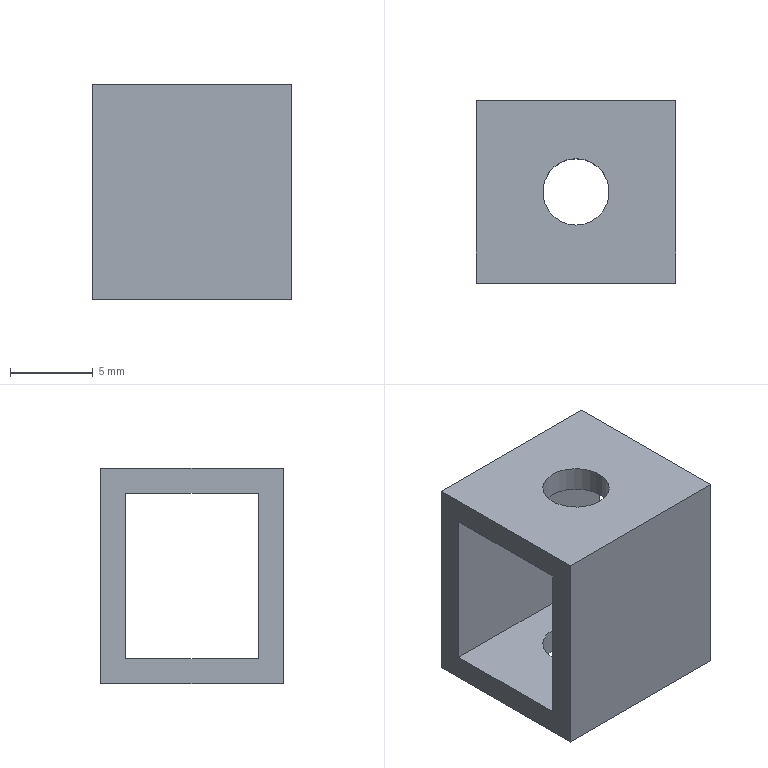Part | STEP file | 1-54.2 | 1 solid | 12 faces | box 12 x 11 x 13 mm | volume 718.301 mm3 | plane 10 | cylinder 2 | commonest cylinder face diameters 4 x2
STEP:
#1=CARTESIAN_POINT('',(0.,0.,0.));
#2=DIRECTION('',(0.,0.,1.));
#3=DIRECTION('',(1.,0.,0.));
#4=AXIS2_PLACEMENT_3D('',#1,#2,#3);
#5=CARTESIAN_POINT('',(6.,-5.5,-6.5));
#6=VERTEX_POINT('',#5);
#7=CARTESIAN_POINT('',(6.,5.5,-6.5));
#8=VERTEX_POINT('',#7);
#9=CARTESIAN_POINT('',(6.,-5.5,-6.5));
#10=DIRECTION('',(0.,1.,0.));
#11=VECTOR('',#10,1.);
#12=LINE('',#9,#11);
#13=CARTESIAN_POINT('',(6.,1.,0.));
#14=DIRECTION('',(1.,0.,0.));
#15=DIRECTION('',(0.,1.,0.));
#16=AXIS2_PLACEMENT_3D('',#13,#14,#15);
#17=PLANE('',#16);
#18=CARTESIAN_POINT('',(-6.5,-6.5));
#19=DIRECTION('',(1.,0.));
#20=VECTOR('',#19,1.);
#21=LINE('',#18,#20);
#22=(GEOMETRIC_REPRESENTATION_CONTEXT(2)PARAMETRIC_REPRESENTATION_CONTEXT()REPRESENTATION_CONTEXT('',''));
#23=DEFINITIONAL_REPRESENTATION('',(#21),#22);
#24=PCURVE('',#17,#23);
#25=CARTESIAN_POINT('',(0.,0.,-6.5));
#26=DIRECTION('',(0.,0.,1.));
#27=DIRECTION('',(0.,1.,0.));
#28=AXIS2_PLACEMENT_3D('',#25,#26,#27);
#29=PLANE('',#28);
#30=CARTESIAN_POINT('',(-5.5,-6.));
#31=DIRECTION('',(1.,0.));
#32=VECTOR('',#31,1.);
#33=LINE('',#30,#32);
#34=(GEOMETRIC_REPRESENTATION_CONTEXT(2)PARAMETRIC_REPRESENTATION_CONTEXT()REPRESENTATION_CONTEXT('',''));
#35=DEFINITIONAL_REPRESENTATION('',(#33),#34);
#36=PCURVE('',#29,#35);
#37=SURFACE_CURVE('',#12,(#24,#36),.PCURVE_S1.);
#38=EDGE_CURVE('',#6,#8,#37,.T.);
#39=ORIENTED_EDGE('',*,*,#38,.T.);
#40=CARTESIAN_POINT('',(6.,5.5,6.5));
#41=VERTEX_POINT('',#40);
#42=CARTESIAN_POINT('',(6.,5.5,-6.5));
#43=DIRECTION('',(0.,0.,1.));
#44=VECTOR('',#43,1.);
#45=LINE('',#42,#44);
#46=CARTESIAN_POINT('',(4.5,-6.5));
#47=DIRECTION('',(0.,1.));
#48=VECTOR('',#47,1.);
#49=LINE('',#46,#48);
#50=(GEOMETRIC_REPRESENTATION_CONTEXT(2)PARAMETRIC_REPRESENTATION_CONTEXT()REPRESENTATION_CONTEXT('',''));
#51=DEFINITIONAL_REPRESENTATION('',(#49),#50);
#52=PCURVE('',#17,#51);
#53=CARTESIAN_POINT('',(0.,5.5,0.));
#54=DIRECTION('',(0.,-1.,0.));
#55=DIRECTION('',(0.,0.,1.));
#56=AXIS2_PLACEMENT_3D('',#53,#54,#55);
#57=PLANE('',#56);
#58=CARTESIAN_POINT('',(-6.5,-6.));
#59=DIRECTION('',(1.,0.));
#60=VECTOR('',#59,1.);
#61=LINE('',#58,#60);
#62=(GEOMETRIC_REPRESENTATION_CONTEXT(2)PARAMETRIC_REPRESENTATION_CONTEXT()REPRESENTATION_CONTEXT('',''));
#63=DEFINITIONAL_REPRESENTATION('',(#61),#62);
#64=PCURVE('',#57,#63);
#65=SURFACE_CURVE('',#45,(#52,#64),.PCURVE_S1.);
#66=EDGE_CURVE('',#8,#41,#65,.T.);
#67=ORIENTED_EDGE('',*,*,#66,.T.);
#68=CARTESIAN_POINT('',(6.,-5.5,6.5));
#69=VERTEX_POINT('',#68);
#70=CARTESIAN_POINT('',(6.,5.5,6.5));
#71=DIRECTION('',(0.,-1.,0.));
#72=VECTOR('',#71,1.);
#73=LINE('',#70,#72);
#74=CARTESIAN_POINT('',(4.5,6.5));
#75=DIRECTION('',(-1.,0.));
#76=VECTOR('',#75,1.);
#77=LINE('',#74,#76);
#78=(GEOMETRIC_REPRESENTATION_CONTEXT(2)PARAMETRIC_REPRESENTATION_CONTEXT()REPRESENTATION_CONTEXT('',''));
#79=DEFINITIONAL_REPRESENTATION('',(#77),#78);
#80=PCURVE('',#17,#79);
#81=CARTESIAN_POINT('',(0.,0.,6.5));
#82=DIRECTION('',(0.,0.,-1.));
#83=DIRECTION('',(0.,-1.,0.));
#84=AXIS2_PLACEMENT_3D('',#81,#82,#83);
#85=PLANE('',#84);
#86=CARTESIAN_POINT('',(-5.5,-6.));
#87=DIRECTION('',(1.,0.));
#88=VECTOR('',#87,1.);
#89=LINE('',#86,#88);
#90=(GEOMETRIC_REPRESENTATION_CONTEXT(2)PARAMETRIC_REPRESENTATION_CONTEXT()REPRESENTATION_CONTEXT('',''));
#91=DEFINITIONAL_REPRESENTATION('',(#89),#90);
#92=PCURVE('',#85,#91);
#93=SURFACE_CURVE('',#73,(#80,#92),.PCURVE_S1.);
#94=EDGE_CURVE('',#41,#69,#93,.T.);
#95=ORIENTED_EDGE('',*,*,#94,.T.);
#96=CARTESIAN_POINT('',(6.,-5.5,6.5));
#97=DIRECTION('',(0.,0.,-1.));
#98=VECTOR('',#97,1.);
#99=LINE('',#96,#98);
#100=CARTESIAN_POINT('',(-6.5,6.5));
#101=DIRECTION('',(0.,-1.));
#102=VECTOR('',#101,1.);
#103=LINE('',#100,#102);
#104=(GEOMETRIC_REPRESENTATION_CONTEXT(2)PARAMETRIC_REPRESENTATION_CONTEXT()REPRESENTATION_CONTEXT('',''));
#105=DEFINITIONAL_REPRESENTATION('',(#103),#104);
#106=PCURVE('',#17,#105);
#107=CARTESIAN_POINT('',(0.,-5.5,0.));
#108=DIRECTION('',(0.,1.,0.));
#109=DIRECTION('',(0.,0.,-1.));
#110=AXIS2_PLACEMENT_3D('',#107,#108,#109);
#111=PLANE('',#110);
#112=CARTESIAN_POINT('',(-6.5,-6.));
#113=DIRECTION('',(1.,0.));
#114=VECTOR('',#113,1.);
#115=LINE('',#112,#114);
#116=(GEOMETRIC_REPRESENTATION_CONTEXT(2)PARAMETRIC_REPRESENTATION_CONTEXT()REPRESENTATION_CONTEXT('',''));
#117=DEFINITIONAL_REPRESENTATION('',(#115),#116);
#118=PCURVE('',#111,#117);
#119=SURFACE_CURVE('',#99,(#106,#118),.PCURVE_S1.);
#120=EDGE_CURVE('',#69,#6,#119,.T.);
#121=ORIENTED_EDGE('',*,*,#120,.T.);
#122=EDGE_LOOP('',(#39,#67,#95,#121));
#123=FACE_BOUND('',#122,.T.);
#124=CARTESIAN_POINT('',(6.,-4.,-5.));
#125=VERTEX_POINT('',#124);
#126=CARTESIAN_POINT('',(6.,-4.,5.));
#127=VERTEX_POINT('',#126);
#128=CARTESIAN_POINT('',(6.,-4.,-5.));
#129=DIRECTION('',(0.,0.,1.));
#130=VECTOR('',#129,1.);
#131=LINE('',#128,#130);
#132=CARTESIAN_POINT('',(-5.,-5.));
#133=DIRECTION('',(0.,1.));
#134=VECTOR('',#133,1.);
#135=LINE('',#132,#134);
#136=(GEOMETRIC_REPRESENTATION_CONTEXT(2)PARAMETRIC_REPRESENTATION_CONTEXT()REPRESENTATION_CONTEXT('',''));
#137=DEFINITIONAL_REPRESENTATION('',(#135),#136);
#138=PCURVE('',#17,#137);
#139=CARTESIAN_POINT('',(0.,-4.,0.));
#140=DIRECTION('',(0.,-1.,0.));
#141=DIRECTION('',(0.,0.,1.));
#142=AXIS2_PLACEMENT_3D('',#139,#140,#141);
#143=PLANE('',#142);
#144=CARTESIAN_POINT('',(-5.,-6.));
#145=DIRECTION('',(1.,0.));
#146=VECTOR('',#145,1.);
#147=LINE('',#144,#146);
#148=(GEOMETRIC_REPRESENTATION_CONTEXT(2)PARAMETRIC_REPRESENTATION_CONTEXT()REPRESENTATION_CONTEXT('',''));
#149=DEFINITIONAL_REPRESENTATION('',(#147),#148);
#150=PCURVE('',#143,#149);
#151=SURFACE_CURVE('',#131,(#138,#150),.PCURVE_S1.);
#152=EDGE_CURVE('',#125,#127,#151,.T.);
#153=ORIENTED_EDGE('',*,*,#152,.T.);
#154=CARTESIAN_POINT('',(6.,4.,5.));
#155=VERTEX_POINT('',#154);
#156=CARTESIAN_POINT('',(6.,-4.,5.));
#157=DIRECTION('',(0.,1.,0.));
#158=VECTOR('',#157,1.);
#159=LINE('',#156,#158);
#160=CARTESIAN_POINT('',(-5.,5.));
#161=DIRECTION('',(1.,0.));
#162=VECTOR('',#161,1.);
#163=LINE('',#160,#162);
#164=(GEOMETRIC_REPRESENTATION_CONTEXT(2)PARAMETRIC_REPRESENTATION_CONTEXT()REPRESENTATION_CONTEXT('',''));
#165=DEFINITIONAL_REPRESENTATION('',(#163),#164);
#166=PCURVE('',#17,#165);
#167=CARTESIAN_POINT('',(0.,0.,5.));
#168=DIRECTION('',(0.,0.,1.));
#169=DIRECTION('',(0.,1.,0.));
#170=AXIS2_PLACEMENT_3D('',#167,#168,#169);
#171=PLANE('',#170);
#172=CARTESIAN_POINT('',(-4.,-6.));
#173=DIRECTION('',(1.,0.));
#174=VECTOR('',#173,1.);
#175=LINE('',#172,#174);
#176=(GEOMETRIC_REPRESENTATION_CONTEXT(2)PARAMETRIC_REPRESENTATION_CONTEXT()REPRESENTATION_CONTEXT('',''));
#177=DEFINITIONAL_REPRESENTATION('',(#175),#176);
#178=PCURVE('',#171,#177);
#179=SURFACE_CURVE('',#159,(#166,#178),.PCURVE_S1.);
#180=EDGE_CURVE('',#127,#155,#179,.T.);
#181=ORIENTED_EDGE('',*,*,#180,.T.);
#182=CARTESIAN_POINT('',(6.,4.,-5.));
#183=VERTEX_POINT('',#182);
#184=CARTESIAN_POINT('',(6.,4.,5.));
#185=DIRECTION('',(0.,0.,-1.));
#186=VECTOR('',#185,1.);
#187=LINE('',#184,#186);
#188=CARTESIAN_POINT('',(3.,5.));
#189=DIRECTION('',(0.,-1.));
#190=VECTOR('',#189,1.);
#191=LINE('',#188,#190);
#192=(GEOMETRIC_REPRESENTATION_CONTEXT(2)PARAMETRIC_REPRESENTATION_CONTEXT()REPRESENTATION_CONTEXT('',''));
#193=DEFINITIONAL_REPRESENTATION('',(#191),#192);
#194=PCURVE('',#17,#193);
#195=CARTESIAN_POINT('',(0.,4.,0.));
#196=DIRECTION('',(0.,1.,0.));
#197=DIRECTION('',(0.,0.,-1.));
#198=AXIS2_PLACEMENT_3D('',#195,#196,#197);
#199=PLANE('',#198);
#200=CARTESIAN_POINT('',(-5.,-6.));
#201=DIRECTION('',(1.,0.));
#202=VECTOR('',#201,1.);
#203=LINE('',#200,#202);
#204=(GEOMETRIC_REPRESENTATION_CONTEXT(2)PARAMETRIC_REPRESENTATION_CONTEXT()REPRESENTATION_CONTEXT('',''));
#205=DEFINITIONAL_REPRESENTATION('',(#203),#204);
#206=PCURVE('',#199,#205);
#207=SURFACE_CURVE('',#187,(#194,#206),.PCURVE_S1.);
#208=EDGE_CURVE('',#155,#183,#207,.T.);
#209=ORIENTED_EDGE('',*,*,#208,.T.);
#210=CARTESIAN_POINT('',(6.,4.,-5.));
#211=DIRECTION('',(0.,-1.,0.));
#212=VECTOR('',#211,1.);
#213=LINE('',#210,#212);
#214=CARTESIAN_POINT('',(3.,-5.));
#215=DIRECTION('',(-1.,0.));
#216=VECTOR('',#215,1.);
#217=LINE('',#214,#216);
#218=(GEOMETRIC_REPRESENTATION_CONTEXT(2)PARAMETRIC_REPRESENTATION_CONTEXT()REPRESENTATION_CONTEXT('',''));
#219=DEFINITIONAL_REPRESENTATION('',(#217),#218);
#220=PCURVE('',#17,#219);
#221=CARTESIAN_POINT('',(0.,0.,-5.));
#222=DIRECTION('',(0.,0.,-1.));
#223=DIRECTION('',(0.,-1.,0.));
#224=AXIS2_PLACEMENT_3D('',#221,#222,#223);
#225=PLANE('',#224);
#226=CARTESIAN_POINT('',(-4.,-6.));
#227=DIRECTION('',(1.,0.));
#228=VECTOR('',#227,1.);
#229=LINE('',#226,#228);
#230=(GEOMETRIC_REPRESENTATION_CONTEXT(2)PARAMETRIC_REPRESENTATION_CONTEXT()REPRESENTATION_CONTEXT('',''));
#231=DEFINITIONAL_REPRESENTATION('',(#229),#230);
#232=PCURVE('',#225,#231);
#233=SURFACE_CURVE('',#213,(#220,#232),.PCURVE_S1.);
#234=EDGE_CURVE('',#183,#125,#233,.T.);
#235=ORIENTED_EDGE('',*,*,#234,.T.);
#236=EDGE_LOOP('',(#153,#181,#209,#235));
#237=FACE_BOUND('',#236,.T.);
#238=ADVANCED_FACE('',(#123,#237),#17,.T.);
#239=CARTESIAN_POINT('',(-6.,-5.5,-6.5));
#240=VERTEX_POINT('',#239);
#241=CARTESIAN_POINT('',(-6.,5.5,-6.5));
#242=VERTEX_POINT('',#241);
#243=CARTESIAN_POINT('',(-6.,-5.5,-6.5));
#244=DIRECTION('',(0.,1.,0.));
#245=VECTOR('',#244,1.);
#246=LINE('',#243,#245);
#247=CARTESIAN_POINT('',(-6.,1.,0.));
#248=DIRECTION('',(1.,0.,0.));
#249=DIRECTION('',(0.,1.,0.));
#250=AXIS2_PLACEMENT_3D('',#247,#248,#249);
#251=PLANE('',#250);
#252=CARTESIAN_POINT('',(-6.5,-6.5));
#253=DIRECTION('',(1.,0.));
#254=VECTOR('',#253,1.);
#255=LINE('',#252,#254);
#256=(GEOMETRIC_REPRESENTATION_CONTEXT(2)PARAMETRIC_REPRESENTATION_CONTEXT()REPRESENTATION_CONTEXT('',''));
#257=DEFINITIONAL_REPRESENTATION('',(#255),#256);
#258=PCURVE('',#251,#257);
#259=CARTESIAN_POINT('',(-5.5,6.));
#260=DIRECTION('',(1.,0.));
#261=VECTOR('',#260,1.);
#262=LINE('',#259,#261);
#263=(GEOMETRIC_REPRESENTATION_CONTEXT(2)PARAMETRIC_REPRESENTATION_CONTEXT()REPRESENTATION_CONTEXT('',''));
#264=DEFINITIONAL_REPRESENTATION('',(#262),#263);
#265=PCURVE('',#29,#264);
#266=SURFACE_CURVE('',#246,(#258,#265),.PCURVE_S1.);
#267=EDGE_CURVE('',#240,#242,#266,.T.);
#268=ORIENTED_EDGE('',*,*,#267,.T.);
#269=CARTESIAN_POINT('',(-6.,5.5,6.5));
#270=VERTEX_POINT('',#269);
#271=CARTESIAN_POINT('',(-6.,5.5,-6.5));
#272=DIRECTION('',(0.,0.,1.));
#273=VECTOR('',#272,1.);
#274=LINE('',#271,#273);
#275=CARTESIAN_POINT('',(4.5,-6.5));
#276=DIRECTION('',(0.,1.));
#277=VECTOR('',#276,1.);
#278=LINE('',#275,#277);
#279=(GEOMETRIC_REPRESENTATION_CONTEXT(2)PARAMETRIC_REPRESENTATION_CONTEXT()REPRESENTATION_CONTEXT('',''));
#280=DEFINITIONAL_REPRESENTATION('',(#278),#279);
#281=PCURVE('',#251,#280);
#282=CARTESIAN_POINT('',(-6.5,6.));
#283=DIRECTION('',(1.,0.));
#284=VECTOR('',#283,1.);
#285=LINE('',#282,#284);
#286=(GEOMETRIC_REPRESENTATION_CONTEXT(2)PARAMETRIC_REPRESENTATION_CONTEXT()REPRESENTATION_CONTEXT('',''));
#287=DEFINITIONAL_REPRESENTATION('',(#285),#286);
#288=PCURVE('',#57,#287);
#289=SURFACE_CURVE('',#274,(#281,#288),.PCURVE_S1.);
#290=EDGE_CURVE('',#242,#270,#289,.T.);
#291=ORIENTED_EDGE('',*,*,#290,.T.);
#292=CARTESIAN_POINT('',(-6.,-5.5,6.5));
#293=VERTEX_POINT('',#292);
#294=CARTESIAN_POINT('',(-6.,5.5,6.5));
#295=DIRECTION('',(0.,-1.,0.));
#296=VECTOR('',#295,1.);
#297=LINE('',#294,#296);
#298=CARTESIAN_POINT('',(4.5,6.5));
#299=DIRECTION('',(-1.,0.));
#300=VECTOR('',#299,1.);
#301=LINE('',#298,#300);
#302=(GEOMETRIC_REPRESENTATION_CONTEXT(2)PARAMETRIC_REPRESENTATION_CONTEXT()REPRESENTATION_CONTEXT('',''));
#303=DEFINITIONAL_REPRESENTATION('',(#301),#302);
#304=PCURVE('',#251,#303);
#305=CARTESIAN_POINT('',(-5.5,6.));
#306=DIRECTION('',(1.,0.));
#307=VECTOR('',#306,1.);
#308=LINE('',#305,#307);
#309=(GEOMETRIC_REPRESENTATION_CONTEXT(2)PARAMETRIC_REPRESENTATION_CONTEXT()REPRESENTATION_CONTEXT('',''));
#310=DEFINITIONAL_REPRESENTATION('',(#308),#309);
#311=PCURVE('',#85,#310);
#312=SURFACE_CURVE('',#297,(#304,#311),.PCURVE_S1.);
#313=EDGE_CURVE('',#270,#293,#312,.T.);
#314=ORIENTED_EDGE('',*,*,#313,.T.);
#315=CARTESIAN_POINT('',(-6.,-5.5,6.5));
#316=DIRECTION('',(0.,0.,-1.));
#317=VECTOR('',#316,1.);
#318=LINE('',#315,#317);
#319=CARTESIAN_POINT('',(-6.5,6.5));
#320=DIRECTION('',(0.,-1.));
#321=VECTOR('',#320,1.);
#322=LINE('',#319,#321);
#323=(GEOMETRIC_REPRESENTATION_CONTEXT(2)PARAMETRIC_REPRESENTATION_CONTEXT()REPRESENTATION_CONTEXT('',''));
#324=DEFINITIONAL_REPRESENTATION('',(#322),#323);
#325=PCURVE('',#251,#324);
#326=CARTESIAN_POINT('',(-6.5,6.));
#327=DIRECTION('',(1.,0.));
#328=VECTOR('',#327,1.);
#329=LINE('',#326,#328);
#330=(GEOMETRIC_REPRESENTATION_CONTEXT(2)PARAMETRIC_REPRESENTATION_CONTEXT()REPRESENTATION_CONTEXT('',''));
#331=DEFINITIONAL_REPRESENTATION('',(#329),#330);
#332=PCURVE('',#111,#331);
#333=SURFACE_CURVE('',#318,(#325,#332),.PCURVE_S1.);
#334=EDGE_CURVE('',#293,#240,#333,.T.);
#335=ORIENTED_EDGE('',*,*,#334,.T.);
#336=EDGE_LOOP('',(#268,#291,#314,#335));
#337=FACE_BOUND('',#336,.F.);
#338=CARTESIAN_POINT('',(-6.,-4.,-5.));
#339=VERTEX_POINT('',#338);
#340=CARTESIAN_POINT('',(-6.,-4.,5.));
#341=VERTEX_POINT('',#340);
#342=CARTESIAN_POINT('',(-6.,-4.,-5.));
#343=DIRECTION('',(0.,0.,1.));
#344=VECTOR('',#343,1.);
#345=LINE('',#342,#344);
#346=CARTESIAN_POINT('',(-5.,-5.));
#347=DIRECTION('',(0.,1.));
#348=VECTOR('',#347,1.);
#349=LINE('',#346,#348);
#350=(GEOMETRIC_REPRESENTATION_CONTEXT(2)PARAMETRIC_REPRESENTATION_CONTEXT()REPRESENTATION_CONTEXT('',''));
#351=DEFINITIONAL_REPRESENTATION('',(#349),#350);
#352=PCURVE('',#251,#351);
#353=CARTESIAN_POINT('',(-5.,6.));
#354=DIRECTION('',(1.,0.));
#355=VECTOR('',#354,1.);
#356=LINE('',#353,#355);
#357=(GEOMETRIC_REPRESENTATION_CONTEXT(2)PARAMETRIC_REPRESENTATION_CONTEXT()REPRESENTATION_CONTEXT('',''));
#358=DEFINITIONAL_REPRESENTATION('',(#356),#357);
#359=PCURVE('',#143,#358);
#360=SURFACE_CURVE('',#345,(#352,#359),.PCURVE_S1.);
#361=EDGE_CURVE('',#339,#341,#360,.T.);
#362=ORIENTED_EDGE('',*,*,#361,.T.);
#363=CARTESIAN_POINT('',(-6.,4.,5.));
#364=VERTEX_POINT('',#363);
#365=CARTESIAN_POINT('',(-6.,-4.,5.));
#366=DIRECTION('',(0.,1.,0.));
#367=VECTOR('',#366,1.);
#368=LINE('',#365,#367);
#369=CARTESIAN_POINT('',(-5.,5.));
#370=DIRECTION('',(1.,0.));
#371=VECTOR('',#370,1.);
#372=LINE('',#369,#371);
#373=(GEOMETRIC_REPRESENTATION_CONTEXT(2)PARAMETRIC_REPRESENTATION_CONTEXT()REPRESENTATION_CONTEXT('',''));
#374=DEFINITIONAL_REPRESENTATION('',(#372),#373);
#375=PCURVE('',#251,#374);
#376=CARTESIAN_POINT('',(-4.,6.));
#377=DIRECTION('',(1.,0.));
#378=VECTOR('',#377,1.);
#379=LINE('',#376,#378);
#380=(GEOMETRIC_REPRESENTATION_CONTEXT(2)PARAMETRIC_REPRESENTATION_CONTEXT()REPRESENTATION_CONTEXT('',''));
#381=DEFINITIONAL_REPRESENTATION('',(#379),#380);
#382=PCURVE('',#171,#381);
#383=SURFACE_CURVE('',#368,(#375,#382),.PCURVE_S1.);
#384=EDGE_CURVE('',#341,#364,#383,.T.);
#385=ORIENTED_EDGE('',*,*,#384,.T.);
#386=CARTESIAN_POINT('',(-6.,4.,-5.));
#387=VERTEX_POINT('',#386);
#388=CARTESIAN_POINT('',(-6.,4.,5.));
#389=DIRECTION('',(0.,0.,-1.));
#390=VECTOR('',#389,1.);
#391=LINE('',#388,#390);
#392=CARTESIAN_POINT('',(3.,5.));
#393=DIRECTION('',(0.,-1.));
#394=VECTOR('',#393,1.);
#395=LINE('',#392,#394);
#396=(GEOMETRIC_REPRESENTATION_CONTEXT(2)PARAMETRIC_REPRESENTATION_CONTEXT()REPRESENTATION_CONTEXT('',''));
#397=DEFINITIONAL_REPRESENTATION('',(#395),#396);
#398=PCURVE('',#251,#397);
#399=CARTESIAN_POINT('',(-5.,6.));
#400=DIRECTION('',(1.,0.));
#401=VECTOR('',#400,1.);
#402=LINE('',#399,#401);
#403=(GEOMETRIC_REPRESENTATION_CONTEXT(2)PARAMETRIC_REPRESENTATION_CONTEXT()REPRESENTATION_CONTEXT('',''));
#404=DEFINITIONAL_REPRESENTATION('',(#402),#403);
#405=PCURVE('',#199,#404);
#406=SURFACE_CURVE('',#391,(#398,#405),.PCURVE_S1.);
#407=EDGE_CURVE('',#364,#387,#406,.T.);
#408=ORIENTED_EDGE('',*,*,#407,.T.);
#409=CARTESIAN_POINT('',(-6.,4.,-5.));
#410=DIRECTION('',(0.,-1.,0.));
#411=VECTOR('',#410,1.);
#412=LINE('',#409,#411);
#413=CARTESIAN_POINT('',(3.,-5.));
#414=DIRECTION('',(-1.,0.));
#415=VECTOR('',#414,1.);
#416=LINE('',#413,#415);
#417=(GEOMETRIC_REPRESENTATION_CONTEXT(2)PARAMETRIC_REPRESENTATION_CONTEXT()REPRESENTATION_CONTEXT('',''));
#418=DEFINITIONAL_REPRESENTATION('',(#416),#417);
#419=PCURVE('',#251,#418);
#420=CARTESIAN_POINT('',(-4.,6.));
#421=DIRECTION('',(1.,0.));
#422=VECTOR('',#421,1.);
#423=LINE('',#420,#422);
#424=(GEOMETRIC_REPRESENTATION_CONTEXT(2)PARAMETRIC_REPRESENTATION_CONTEXT()REPRESENTATION_CONTEXT('',''));
#425=DEFINITIONAL_REPRESENTATION('',(#423),#424);
#426=PCURVE('',#225,#425);
#427=SURFACE_CURVE('',#412,(#419,#426),.PCURVE_S1.);
#428=EDGE_CURVE('',#387,#339,#427,.T.);
#429=ORIENTED_EDGE('',*,*,#428,.T.);
#430=EDGE_LOOP('',(#362,#385,#408,#429));
#431=FACE_BOUND('',#430,.F.);
#432=ADVANCED_FACE('',(#337,#431),#251,.F.);
#433=ORIENTED_EDGE('',*,*,#66,.T.);
#434=CARTESIAN_POINT('',(6.,5.5,6.5));
#435=DIRECTION('',(-1.,0.,0.));
#436=VECTOR('',#435,1.);
#437=LINE('',#434,#436);
#438=CARTESIAN_POINT('',(6.5,-6.));
#439=DIRECTION('',(0.,1.));
#440=VECTOR('',#439,1.);
#441=LINE('',#438,#440);
#442=(GEOMETRIC_REPRESENTATION_CONTEXT(2)PARAMETRIC_REPRESENTATION_CONTEXT()REPRESENTATION_CONTEXT('',''));
#443=DEFINITIONAL_REPRESENTATION('',(#441),#442);
#444=PCURVE('',#57,#443);
#445=CARTESIAN_POINT('',(-5.5,-6.));
#446=DIRECTION('',(0.,1.));
#447=VECTOR('',#446,1.);
#448=LINE('',#445,#447);
#449=(GEOMETRIC_REPRESENTATION_CONTEXT(2)PARAMETRIC_REPRESENTATION_CONTEXT()REPRESENTATION_CONTEXT('',''));
#450=DEFINITIONAL_REPRESENTATION('',(#448),#449);
#451=PCURVE('',#85,#450);
#452=SURFACE_CURVE('',#437,(#444,#451),.PCURVE_S1.);
#453=EDGE_CURVE('',#41,#270,#452,.T.);
#454=ORIENTED_EDGE('',*,*,#453,.T.);
#455=ORIENTED_EDGE('',*,*,#290,.F.);
#456=CARTESIAN_POINT('',(6.,5.5,-6.5));
#457=DIRECTION('',(-1.,0.,0.));
#458=VECTOR('',#457,1.);
#459=LINE('',#456,#458);
#460=CARTESIAN_POINT('',(-6.5,-6.));
#461=DIRECTION('',(0.,1.));
#462=VECTOR('',#461,1.);
#463=LINE('',#460,#462);
#464=(GEOMETRIC_REPRESENTATION_CONTEXT(2)PARAMETRIC_REPRESENTATION_CONTEXT()REPRESENTATION_CONTEXT('',''));
#465=DEFINITIONAL_REPRESENTATION('',(#463),#464);
#466=PCURVE('',#57,#465);
#467=CARTESIAN_POINT('',(5.5,-6.));
#468=DIRECTION('',(0.,1.));
#469=VECTOR('',#468,1.);
#470=LINE('',#467,#469);
#471=(GEOMETRIC_REPRESENTATION_CONTEXT(2)PARAMETRIC_REPRESENTATION_CONTEXT()REPRESENTATION_CONTEXT('',''));
#472=DEFINITIONAL_REPRESENTATION('',(#470),#471);
#473=PCURVE('',#29,#472);
#474=SURFACE_CURVE('',#459,(#466,#473),.PCURVE_S1.);
#475=EDGE_CURVE('',#8,#242,#474,.T.);
#476=ORIENTED_EDGE('',*,*,#475,.F.);
#477=EDGE_LOOP('',(#433,#454,#455,#476));
#478=FACE_BOUND('',#477,.F.);
#479=ADVANCED_FACE('',(#478),#57,.F.);
#480=ORIENTED_EDGE('',*,*,#120,.T.);
#481=CARTESIAN_POINT('',(6.,-5.5,-6.5));
#482=DIRECTION('',(-1.,0.,0.));
#483=VECTOR('',#482,1.);
#484=LINE('',#481,#483);
#485=CARTESIAN_POINT('',(6.5,-6.));
#486=DIRECTION('',(0.,1.));
#487=VECTOR('',#486,1.);
#488=LINE('',#485,#487);
#489=(GEOMETRIC_REPRESENTATION_CONTEXT(2)PARAMETRIC_REPRESENTATION_CONTEXT()REPRESENTATION_CONTEXT('',''));
#490=DEFINITIONAL_REPRESENTATION('',(#488),#489);
#491=PCURVE('',#111,#490);
#492=CARTESIAN_POINT('',(-5.5,-6.));
#493=DIRECTION('',(0.,1.));
#494=VECTOR('',#493,1.);
#495=LINE('',#492,#494);
#496=(GEOMETRIC_REPRESENTATION_CONTEXT(2)PARAMETRIC_REPRESENTATION_CONTEXT()REPRESENTATION_CONTEXT('',''));
#497=DEFINITIONAL_REPRESENTATION('',(#495),#496);
#498=PCURVE('',#29,#497);
#499=SURFACE_CURVE('',#484,(#491,#498),.PCURVE_S1.);
#500=EDGE_CURVE('',#6,#240,#499,.T.);
#501=ORIENTED_EDGE('',*,*,#500,.T.);
#502=ORIENTED_EDGE('',*,*,#334,.F.);
#503=CARTESIAN_POINT('',(6.,-5.5,6.5));
#504=DIRECTION('',(-1.,0.,0.));
#505=VECTOR('',#504,1.);
#506=LINE('',#503,#505);
#507=CARTESIAN_POINT('',(-6.5,-6.));
#508=DIRECTION('',(0.,1.));
#509=VECTOR('',#508,1.);
#510=LINE('',#507,#509);
#511=(GEOMETRIC_REPRESENTATION_CONTEXT(2)PARAMETRIC_REPRESENTATION_CONTEXT()REPRESENTATION_CONTEXT('',''));
#512=DEFINITIONAL_REPRESENTATION('',(#510),#511);
#513=PCURVE('',#111,#512);
#514=CARTESIAN_POINT('',(5.5,-6.));
#515=DIRECTION('',(0.,1.));
#516=VECTOR('',#515,1.);
#517=LINE('',#514,#516);
#518=(GEOMETRIC_REPRESENTATION_CONTEXT(2)PARAMETRIC_REPRESENTATION_CONTEXT()REPRESENTATION_CONTEXT('',''));
#519=DEFINITIONAL_REPRESENTATION('',(#517),#518);
#520=PCURVE('',#85,#519);
#521=SURFACE_CURVE('',#506,(#513,#520),.PCURVE_S1.);
#522=EDGE_CURVE('',#69,#293,#521,.T.);
#523=ORIENTED_EDGE('',*,*,#522,.F.);
#524=EDGE_LOOP('',(#480,#501,#502,#523));
#525=FACE_BOUND('',#524,.F.);
#526=ADVANCED_FACE('',(#525),#111,.F.);
#527=ORIENTED_EDGE('',*,*,#152,.T.);
#528=CARTESIAN_POINT('',(6.,-4.,5.));
#529=DIRECTION('',(-1.,0.,0.));
#530=VECTOR('',#529,1.);
#531=LINE('',#528,#530);
#532=CARTESIAN_POINT('',(5.,-6.));
#533=DIRECTION('',(0.,1.));
#534=VECTOR('',#533,1.);
#535=LINE('',#532,#534);
#536=(GEOMETRIC_REPRESENTATION_CONTEXT(2)PARAMETRIC_REPRESENTATION_CONTEXT()REPRESENTATION_CONTEXT('',''));
#537=DEFINITIONAL_REPRESENTATION('',(#535),#536);
#538=PCURVE('',#143,#537);
#539=CARTESIAN_POINT('',(-4.,-6.));
#540=DIRECTION('',(0.,1.));
#541=VECTOR('',#540,1.);
#542=LINE('',#539,#541);
#543=(GEOMETRIC_REPRESENTATION_CONTEXT(2)PARAMETRIC_REPRESENTATION_CONTEXT()REPRESENTATION_CONTEXT('',''));
#544=DEFINITIONAL_REPRESENTATION('',(#542),#543);
#545=PCURVE('',#171,#544);
#546=SURFACE_CURVE('',#531,(#538,#545),.PCURVE_S1.);
#547=EDGE_CURVE('',#127,#341,#546,.T.);
#548=ORIENTED_EDGE('',*,*,#547,.T.);
#549=ORIENTED_EDGE('',*,*,#361,.F.);
#550=CARTESIAN_POINT('',(6.,-4.,-5.));
#551=DIRECTION('',(-1.,0.,0.));
#552=VECTOR('',#551,1.);
#553=LINE('',#550,#552);
#554=CARTESIAN_POINT('',(-5.,-6.));
#555=DIRECTION('',(0.,1.));
#556=VECTOR('',#555,1.);
#557=LINE('',#554,#556);
#558=(GEOMETRIC_REPRESENTATION_CONTEXT(2)PARAMETRIC_REPRESENTATION_CONTEXT()REPRESENTATION_CONTEXT('',''));
#559=DEFINITIONAL_REPRESENTATION('',(#557),#558);
#560=PCURVE('',#143,#559);
#561=CARTESIAN_POINT('',(4.,-6.));
#562=DIRECTION('',(0.,1.));
#563=VECTOR('',#562,1.);
#564=LINE('',#561,#563);
#565=(GEOMETRIC_REPRESENTATION_CONTEXT(2)PARAMETRIC_REPRESENTATION_CONTEXT()REPRESENTATION_CONTEXT('',''));
#566=DEFINITIONAL_REPRESENTATION('',(#564),#565);
#567=PCURVE('',#225,#566);
#568=SURFACE_CURVE('',#553,(#560,#567),.PCURVE_S1.);
#569=EDGE_CURVE('',#125,#339,#568,.T.);
#570=ORIENTED_EDGE('',*,*,#569,.F.);
#571=EDGE_LOOP('',(#527,#548,#549,#570));
#572=FACE_BOUND('',#571,.F.);
#573=ADVANCED_FACE('',(#572),#143,.F.);
#574=ORIENTED_EDGE('',*,*,#208,.T.);
#575=CARTESIAN_POINT('',(6.,4.,-5.));
#576=DIRECTION('',(-1.,0.,0.));
#577=VECTOR('',#576,1.);
#578=LINE('',#575,#577);
#579=CARTESIAN_POINT('',(5.,-6.));
#580=DIRECTION('',(0.,1.));
#581=VECTOR('',#580,1.);
#582=LINE('',#579,#581);
#583=(GEOMETRIC_REPRESENTATION_CONTEXT(2)PARAMETRIC_REPRESENTATION_CONTEXT()REPRESENTATION_CONTEXT('',''));
#584=DEFINITIONAL_REPRESENTATION('',(#582),#583);
#585=PCURVE('',#199,#584);
#586=CARTESIAN_POINT('',(-4.,-6.));
#587=DIRECTION('',(0.,1.));
#588=VECTOR('',#587,1.);
#589=LINE('',#586,#588);
#590=(GEOMETRIC_REPRESENTATION_CONTEXT(2)PARAMETRIC_REPRESENTATION_CONTEXT()REPRESENTATION_CONTEXT('',''));
#591=DEFINITIONAL_REPRESENTATION('',(#589),#590);
#592=PCURVE('',#225,#591);
#593=SURFACE_CURVE('',#578,(#585,#592),.PCURVE_S1.);
#594=EDGE_CURVE('',#183,#387,#593,.T.);
#595=ORIENTED_EDGE('',*,*,#594,.T.);
#596=ORIENTED_EDGE('',*,*,#407,.F.);
#597=CARTESIAN_POINT('',(6.,4.,5.));
#598=DIRECTION('',(-1.,0.,0.));
#599=VECTOR('',#598,1.);
#600=LINE('',#597,#599);
#601=CARTESIAN_POINT('',(-5.,-6.));
#602=DIRECTION('',(0.,1.));
#603=VECTOR('',#602,1.);
#604=LINE('',#601,#603);
#605=(GEOMETRIC_REPRESENTATION_CONTEXT(2)PARAMETRIC_REPRESENTATION_CONTEXT()REPRESENTATION_CONTEXT('',''));
#606=DEFINITIONAL_REPRESENTATION('',(#604),#605);
#607=PCURVE('',#199,#606);
#608=CARTESIAN_POINT('',(4.,-6.));
#609=DIRECTION('',(0.,1.));
#610=VECTOR('',#609,1.);
#611=LINE('',#608,#610);
#612=(GEOMETRIC_REPRESENTATION_CONTEXT(2)PARAMETRIC_REPRESENTATION_CONTEXT()REPRESENTATION_CONTEXT('',''));
#613=DEFINITIONAL_REPRESENTATION('',(#611),#612);
#614=PCURVE('',#171,#613);
#615=SURFACE_CURVE('',#600,(#607,#614),.PCURVE_S1.);
#616=EDGE_CURVE('',#155,#364,#615,.T.);
#617=ORIENTED_EDGE('',*,*,#616,.F.);
#618=EDGE_LOOP('',(#574,#595,#596,#617));
#619=FACE_BOUND('',#618,.F.);
#620=ADVANCED_FACE('',(#619),#199,.F.);
#621=ORIENTED_EDGE('',*,*,#38,.T.);
#622=ORIENTED_EDGE('',*,*,#475,.T.);
#623=ORIENTED_EDGE('',*,*,#267,.F.);
#624=ORIENTED_EDGE('',*,*,#500,.F.);
#625=EDGE_LOOP('',(#621,#622,#623,#624));
#626=FACE_BOUND('',#625,.F.);
#627=CARTESIAN_POINT('',(0.,2.,-6.5));
#628=VERTEX_POINT('',#627);
#629=CARTESIAN_POINT('',(0.,0.,-6.5));
#630=DIRECTION('',(0.,0.,1.));
#631=DIRECTION('',(0.,1.,0.));
#632=AXIS2_PLACEMENT_3D('',#629,#630,#631);
#633=CIRCLE('',#632,2.);
#634=CARTESIAN_POINT('',(0.,0.));
#635=DIRECTION('',(1.,0.));
#636=AXIS2_PLACEMENT_2D('',#634,#635);
#637=CIRCLE('',#636,2.);
#638=(GEOMETRIC_REPRESENTATION_CONTEXT(2)PARAMETRIC_REPRESENTATION_CONTEXT()REPRESENTATION_CONTEXT('',''));
#639=DEFINITIONAL_REPRESENTATION('',(#637),#638);
#640=PCURVE('',#29,#639);
#641=CARTESIAN_POINT('',(0.,0.,6.5));
#642=DIRECTION('',(0.,0.,-1.));
#643=DIRECTION('',(0.,1.,0.));
#644=AXIS2_PLACEMENT_3D('',#641,#642,#643);
#645=CYLINDRICAL_SURFACE('',#644,2.);
#646=CARTESIAN_POINT('',(6.283,13.));
#647=DIRECTION('',(-1.,0.));
#648=VECTOR('',#647,1.);
#649=LINE('',#646,#648);
#650=(GEOMETRIC_REPRESENTATION_CONTEXT(2)PARAMETRIC_REPRESENTATION_CONTEXT()REPRESENTATION_CONTEXT('',''));
#651=DEFINITIONAL_REPRESENTATION('',(#649),#650);
#652=PCURVE('',#645,#651);
#653=SURFACE_CURVE('',#633,(#640,#652),.PCURVE_S1.);
#654=EDGE_CURVE('',#628,#628,#653,.T.);
#655=ORIENTED_EDGE('',*,*,#654,.F.);
#656=EDGE_LOOP('',(#655));
#657=FACE_BOUND('',#656,.F.);
#658=ADVANCED_FACE('',(#626,#657),#29,.F.);
#659=ORIENTED_EDGE('',*,*,#94,.T.);
#660=ORIENTED_EDGE('',*,*,#522,.T.);
#661=ORIENTED_EDGE('',*,*,#313,.F.);
#662=ORIENTED_EDGE('',*,*,#453,.F.);
#663=EDGE_LOOP('',(#659,#660,#661,#662));
#664=FACE_BOUND('',#663,.F.);
#665=CARTESIAN_POINT('',(0.,2.,6.5));
#666=VERTEX_POINT('',#665);
#667=CARTESIAN_POINT('',(0.,0.,6.5));
#668=DIRECTION('',(0.,0.,1.));
#669=DIRECTION('',(0.,1.,0.));
#670=AXIS2_PLACEMENT_3D('',#667,#668,#669);
#671=CIRCLE('',#670,2.);
#672=CARTESIAN_POINT('',(-2.,0.));
#673=CARTESIAN_POINT('',(-2.,3.464));
#674=CARTESIAN_POINT('',(1.,1.732));
#675=CARTESIAN_POINT('',(4.,0.));
#676=CARTESIAN_POINT('',(1.,-1.732));
#677=CARTESIAN_POINT('',(-2.,-3.464));
#678=CARTESIAN_POINT('',(-2.,0.));
#679=(BOUNDED_CURVE()B_SPLINE_CURVE(2,(#672,#673,#674,#675,#676,#677,#678),.UNSPECIFIED.,.T.,.F.)B_SPLINE_CURVE_WITH_KNOTS((1,2,2,2,2,1),(-2.094,0.,2.094,4.189,6.283,8.378),.UNSPECIFIED.)CURVE()GEOMETRIC_REPRESENTATION_ITEM()RATIONAL_B_SPLINE_CURVE((1.,0.5,1.,0.5,1.,0.5,1.))REPRESENTATION_ITEM(''));
#680=(GEOMETRIC_REPRESENTATION_CONTEXT(2)PARAMETRIC_REPRESENTATION_CONTEXT()REPRESENTATION_CONTEXT('',''));
#681=DEFINITIONAL_REPRESENTATION('',(#679),#680);
#682=PCURVE('',#85,#681);
#683=CARTESIAN_POINT('',(0.,0.,6.5));
#684=DIRECTION('',(0.,0.,-1.));
#685=DIRECTION('',(0.,1.,0.));
#686=AXIS2_PLACEMENT_3D('',#683,#684,#685);
#687=CYLINDRICAL_SURFACE('',#686,2.);
#688=CARTESIAN_POINT('',(6.283,0.));
#689=DIRECTION('',(-1.,0.));
#690=VECTOR('',#689,1.);
#691=LINE('',#688,#690);
#692=(GEOMETRIC_REPRESENTATION_CONTEXT(2)PARAMETRIC_REPRESENTATION_CONTEXT()REPRESENTATION_CONTEXT('',''));
#693=DEFINITIONAL_REPRESENTATION('',(#691),#692);
#694=PCURVE('',#687,#693);
#695=SURFACE_CURVE('',#671,(#682,#694),.PCURVE_S1.);
#696=EDGE_CURVE('',#666,#666,#695,.T.);
#697=ORIENTED_EDGE('',*,*,#696,.T.);
#698=EDGE_LOOP('',(#697));
#699=FACE_BOUND('',#698,.F.);
#700=ADVANCED_FACE('',(#664,#699),#85,.F.);
#701=ORIENTED_EDGE('',*,*,#180,.T.);
#702=ORIENTED_EDGE('',*,*,#616,.T.);
#703=ORIENTED_EDGE('',*,*,#384,.F.);
#704=ORIENTED_EDGE('',*,*,#547,.F.);
#705=EDGE_LOOP('',(#701,#702,#703,#704));
#706=FACE_BOUND('',#705,.F.);
#707=CARTESIAN_POINT('',(0.,2.,5.));
#708=VERTEX_POINT('',#707);
#709=CARTESIAN_POINT('',(0.,0.,5.));
#710=DIRECTION('',(0.,0.,-1.));
#711=DIRECTION('',(0.,1.,0.));
#712=AXIS2_PLACEMENT_3D('',#709,#710,#711);
#713=CIRCLE('',#712,2.);
#714=CARTESIAN_POINT('',(2.,0.));
#715=CARTESIAN_POINT('',(2.,-3.464));
#716=CARTESIAN_POINT('',(-1.,-1.732));
#717=CARTESIAN_POINT('',(-4.,0.));
#718=CARTESIAN_POINT('',(-1.,1.732));
#719=CARTESIAN_POINT('',(2.,3.464));
#720=CARTESIAN_POINT('',(2.,0.));
#721=(BOUNDED_CURVE()B_SPLINE_CURVE(2,(#714,#715,#716,#717,#718,#719,#720),.UNSPECIFIED.,.T.,.F.)B_SPLINE_CURVE_WITH_KNOTS((1,2,2,2,2,1),(-2.094,0.,2.094,4.189,6.283,8.378),.UNSPECIFIED.)CURVE()GEOMETRIC_REPRESENTATION_ITEM()RATIONAL_B_SPLINE_CURVE((1.,0.5,1.,0.5,1.,0.5,1.))REPRESENTATION_ITEM(''));
#722=(GEOMETRIC_REPRESENTATION_CONTEXT(2)PARAMETRIC_REPRESENTATION_CONTEXT()REPRESENTATION_CONTEXT('',''));
#723=DEFINITIONAL_REPRESENTATION('',(#721),#722);
#724=PCURVE('',#171,#723);
#725=CARTESIAN_POINT('',(0.,1.5));
#726=DIRECTION('',(1.,0.));
#727=VECTOR('',#726,1.);
#728=LINE('',#725,#727);
#729=(GEOMETRIC_REPRESENTATION_CONTEXT(2)PARAMETRIC_REPRESENTATION_CONTEXT()REPRESENTATION_CONTEXT('',''));
#730=DEFINITIONAL_REPRESENTATION('',(#728),#729);
#731=PCURVE('',#687,#730);
#732=SURFACE_CURVE('',#713,(#724,#731),.PCURVE_S1.);
#733=EDGE_CURVE('',#708,#708,#732,.T.);
#734=ORIENTED_EDGE('',*,*,#733,.T.);
#735=EDGE_LOOP('',(#734));
#736=FACE_BOUND('',#735,.F.);
#737=ADVANCED_FACE('',(#706,#736),#171,.F.);
#738=ORIENTED_EDGE('',*,*,#234,.T.);
#739=ORIENTED_EDGE('',*,*,#569,.T.);
#740=ORIENTED_EDGE('',*,*,#428,.F.);
#741=ORIENTED_EDGE('',*,*,#594,.F.);
#742=EDGE_LOOP('',(#738,#739,#740,#741));
#743=FACE_BOUND('',#742,.F.);
#744=CARTESIAN_POINT('',(0.,2.,-5.));
#745=VERTEX_POINT('',#744);
#746=CARTESIAN_POINT('',(0.,0.,-5.));
#747=DIRECTION('',(0.,0.,1.));
#748=DIRECTION('',(0.,1.,0.));
#749=AXIS2_PLACEMENT_3D('',#746,#747,#748);
#750=CIRCLE('',#749,2.);
#751=CARTESIAN_POINT('',(-2.,0.));
#752=CARTESIAN_POINT('',(-2.,3.464));
#753=CARTESIAN_POINT('',(1.,1.732));
#754=CARTESIAN_POINT('',(4.,0.));
#755=CARTESIAN_POINT('',(1.,-1.732));
#756=CARTESIAN_POINT('',(-2.,-3.464));
#757=CARTESIAN_POINT('',(-2.,0.));
#758=(BOUNDED_CURVE()B_SPLINE_CURVE(2,(#751,#752,#753,#754,#755,#756,#757),.UNSPECIFIED.,.T.,.F.)B_SPLINE_CURVE_WITH_KNOTS((1,2,2,2,2,1),(-2.094,0.,2.094,4.189,6.283,8.378),.UNSPECIFIED.)CURVE()GEOMETRIC_REPRESENTATION_ITEM()RATIONAL_B_SPLINE_CURVE((1.,0.5,1.,0.5,1.,0.5,1.))REPRESENTATION_ITEM(''));
#759=(GEOMETRIC_REPRESENTATION_CONTEXT(2)PARAMETRIC_REPRESENTATION_CONTEXT()REPRESENTATION_CONTEXT('',''));
#760=DEFINITIONAL_REPRESENTATION('',(#758),#759);
#761=PCURVE('',#225,#760);
#762=CARTESIAN_POINT('',(6.283,11.5));
#763=DIRECTION('',(-1.,0.));
#764=VECTOR('',#763,1.);
#765=LINE('',#762,#764);
#766=(GEOMETRIC_REPRESENTATION_CONTEXT(2)PARAMETRIC_REPRESENTATION_CONTEXT()REPRESENTATION_CONTEXT('',''));
#767=DEFINITIONAL_REPRESENTATION('',(#765),#766);
#768=PCURVE('',#645,#767);
#769=SURFACE_CURVE('',#750,(#761,#768),.PCURVE_S1.);
#770=EDGE_CURVE('',#745,#745,#769,.T.);
#771=ORIENTED_EDGE('',*,*,#770,.T.);
#772=EDGE_LOOP('',(#771));
#773=FACE_BOUND('',#772,.F.);
#774=ADVANCED_FACE('',(#743,#773),#225,.F.);
#775=CARTESIAN_POINT('',(0.,2.,-5.));
#776=DIRECTION('',(0.,0.,-1.));
#777=VECTOR('',#776,1.);
#778=LINE('',#775,#777);
#779=CARTESIAN_POINT('',(0.,11.5));
#780=DIRECTION('',(0.,1.));
#781=VECTOR('',#780,1.);
#782=LINE('',#779,#781);
#783=(GEOMETRIC_REPRESENTATION_CONTEXT(2)PARAMETRIC_REPRESENTATION_CONTEXT()REPRESENTATION_CONTEXT('',''));
#784=DEFINITIONAL_REPRESENTATION('',(#782),#783);
#785=PCURVE('',#645,#784);
#786=CARTESIAN_POINT('',(6.283,11.5));
#787=DIRECTION('',(0.,1.));
#788=VECTOR('',#787,1.);
#789=LINE('',#786,#788);
#790=(GEOMETRIC_REPRESENTATION_CONTEXT(2)PARAMETRIC_REPRESENTATION_CONTEXT()REPRESENTATION_CONTEXT('',''));
#791=DEFINITIONAL_REPRESENTATION('',(#789),#790);
#792=PCURVE('',#645,#791);
#793=SEAM_CURVE('',#778,(#785,#792),.PCURVE_S1.);
#794=EDGE_CURVE('',#745,#628,#793,.T.);
#795=ORIENTED_EDGE('',*,*,#794,.F.);
#796=ORIENTED_EDGE('',*,*,#770,.F.);
#797=ORIENTED_EDGE('',*,*,#794,.T.);
#798=ORIENTED_EDGE('',*,*,#654,.T.);
#799=EDGE_LOOP('',(#795,#796,#797,#798));
#800=FACE_BOUND('',#799,.F.);
#801=ADVANCED_FACE('',(#800),#645,.F.);
#802=CARTESIAN_POINT('',(0.,2.,6.5));
#803=DIRECTION('',(0.,0.,-1.));
#804=VECTOR('',#803,1.);
#805=LINE('',#802,#804);
#806=CARTESIAN_POINT('',(6.283,0.));
#807=DIRECTION('',(0.,1.));
#808=VECTOR('',#807,1.);
#809=LINE('',#806,#808);
#810=(GEOMETRIC_REPRESENTATION_CONTEXT(2)PARAMETRIC_REPRESENTATION_CONTEXT()REPRESENTATION_CONTEXT('',''));
#811=DEFINITIONAL_REPRESENTATION('',(#809),#810);
#812=PCURVE('',#687,#811);
#813=CARTESIAN_POINT('',(0.,0.));
#814=DIRECTION('',(0.,1.));
#815=VECTOR('',#814,1.);
#816=LINE('',#813,#815);
#817=(GEOMETRIC_REPRESENTATION_CONTEXT(2)PARAMETRIC_REPRESENTATION_CONTEXT()REPRESENTATION_CONTEXT('',''));
#818=DEFINITIONAL_REPRESENTATION('',(#816),#817);
#819=PCURVE('',#687,#818);
#820=SEAM_CURVE('',#805,(#812,#819),.PCURVE_S1.);
#821=EDGE_CURVE('',#666,#708,#820,.T.);
#822=ORIENTED_EDGE('',*,*,#821,.T.);
#823=ORIENTED_EDGE('',*,*,#733,.F.);
#824=ORIENTED_EDGE('',*,*,#821,.F.);
#825=ORIENTED_EDGE('',*,*,#696,.F.);
#826=EDGE_LOOP('',(#822,#823,#824,#825));
#827=FACE_BOUND('',#826,.F.);
#828=ADVANCED_FACE('',(#827),#687,.F.);
#829=CLOSED_SHELL('',(#238,#432,#479,#526,#573,#620,#658,#700,#737,#774,#801,#828));
#830=MANIFOLD_SOLID_BREP('',#829);
#831=(LENGTH_UNIT()NAMED_UNIT(*)SI_UNIT(.MILLI.,.METRE.));
#832=UNCERTAINTY_MEASURE_WITH_UNIT(LENGTH_MEASURE(0.0000001),#831,'','');
#833=(NAMED_UNIT(*)PLANE_ANGLE_UNIT()SI_UNIT($,.RADIAN.));
#834=(NAMED_UNIT(*)SI_UNIT($,.STERADIAN.)SOLID_ANGLE_UNIT());
#835=(GEOMETRIC_REPRESENTATION_CONTEXT(3)GLOBAL_UNCERTAINTY_ASSIGNED_CONTEXT((#832))GLOBAL_UNIT_ASSIGNED_CONTEXT((#831,#833,#834))REPRESENTATION_CONTEXT('',''));
#836=ADVANCED_BREP_SHAPE_REPRESENTATION('',(#4,#830),#835);